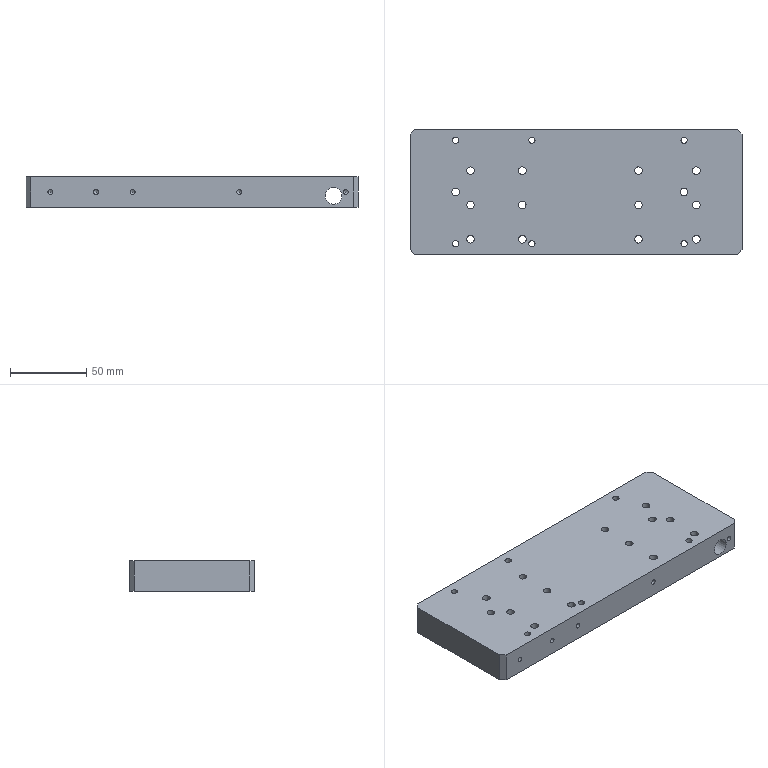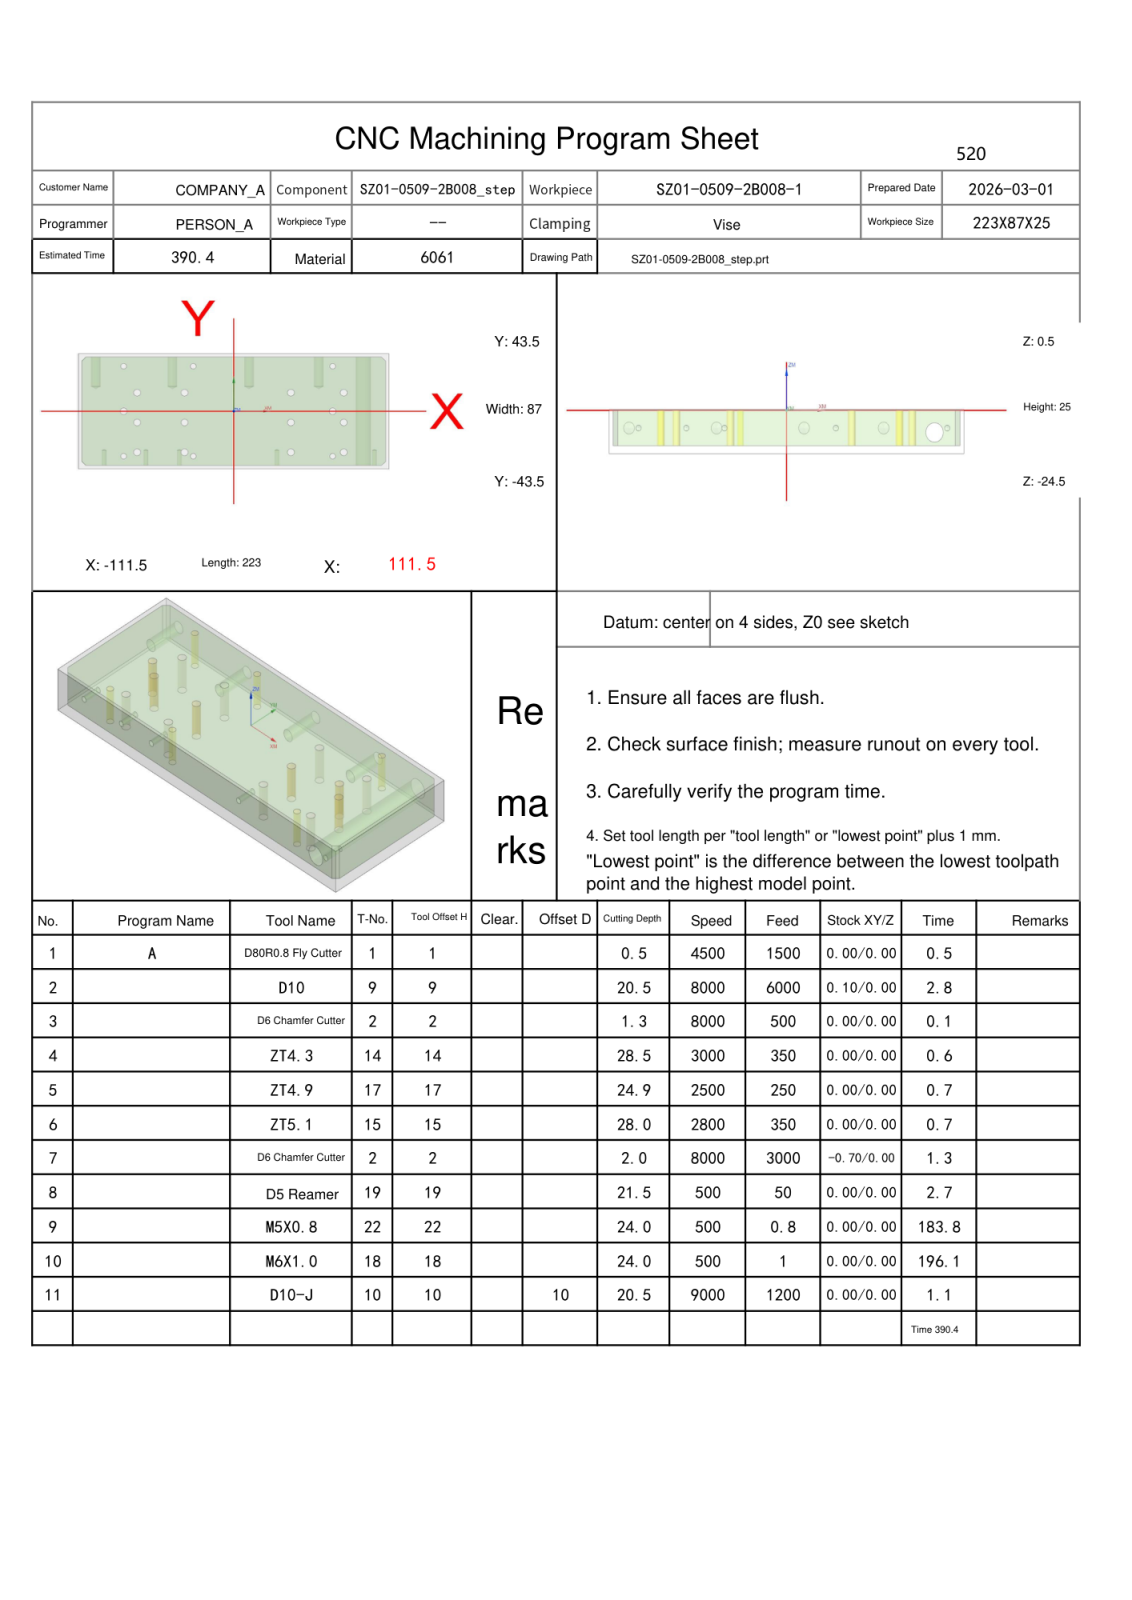NC program | NX | posted by the shop | part box 218 x 82 x 20 mm
Whole program:
%
O0001
(Machine time: 756.44 MIN)
(===Total Tool:10===)
(T1=D80R0.8 Fly Cutter D=80.  R=0.8  D-  H01 Z=0.    )
(T9=D10     D=10.  R=0.   D-  H09 Z=-20.  )
(T2=D6 Chamfer Cutter   D=6.   R=0.   D-  H02 Z=-1.5  )
(T14=ZT4.3  D=4.3  DR_a=118 D-  H14 Z=-28.  )
(T17=ZT4.9  D=4.9  DR_a=120 D-  H17 Z=-24.41)
(T15=ZT5.1  D=5.1  DR_a=118 D-  H15 Z=-27.53)
(T19=D5 Reamer   D=5.   DR_a=180 D-  H19 Z=-21.  )
(T22=M5X0.8 D=4.2  DR_a=180 D-  H22 Z=-23.5 )
(T18=M6X1.0 D=5.   DR_a=180 D-  H18 Z=-23.5 )
(T10=D10-J  D=10.  R=0.   D10 H10 Z=-20.  )
G80 G90 G17 G49 G40
G91 G28 Z0
M01
N1 T01 M06
(D80R0.8 Fly Cutter  D=80. R=0.8 H=01 ce=0.00 di=0.00)
G00 G90 G54 X-154. Y27. M03 S4500
G43 H01 Z50.
M08
Z2.
G01 Z0.0 F1500.
X-149.
X149.
Y-27.
X-149.
X-154.
Z2.
G00 Z50.
G91 G28 Z0.0
M05
M09
G91 G28 Z0.0
M01
N2 T09 M06
(D10  D=10. R=0. H=09 ce=0.10 di=0.00)
G00 G90 G54 X0.0 Y46.1 M03 S8000
G43 H09 Z50.
M08
Z.5
G01 X106. Z.366 F6000.
G02 X109.606 Y44.606 Z.361 I0.0 J-5.1
G01 X112.606 Y41.606 Z.356
G02 X114.1 Y38. Z.351 I-3.606 J-3.606
G01 Y-38. Z.255
G02 X112.606 Y-41.606 Z.25 I-5.1 J0.0
G01 X109.606 Y-44.606 Z.245
G02 X106. Y-46.1 Z.239 I-3.606 J3.606
G01 X-106. Z-.028
G02 X-109.606 Y-44.606 Z-.033 I0.0 J5.1
G01 X-112.606 Y-41.606 Z-.038
G02 X-114.1 Y-38. Z-.043 I3.606 J3.606
G01 Y38. Z-.139
G02 X-112.606 Y41.606 Z-.144 I5.1 J0.0
G01 X-109.606 Y44.606 Z-.15
G02 X-107.242 Y45.946 Z-.153 I3.606 J-3.606
X-106. Y46.1 Z-.155 I1.242 J-4.946
G01 X106. Z-.422
G02 X109.606 Y44.606 Z-.427 I0.0 J-5.1
G01 X112.606 Y41.606 Z-.433
G02 X114.1 Y38. Z-.438 I-3.606 J-3.606
G01 Y-38. Z-.534
G02 X112.606 Y-41.606 Z-.539 I-5.1 J0.0
G01 X109.606 Y-44.606 Z-.544
G02 X106. Y-46.1 Z-.549 I-3.606 J3.606
G01 X-106. Z-.816
G02 X-109.606 Y-44.606 Z-.821 I0.0 J5.1
G01 X-112.606 Y-41.606 Z-.827
G02 X-114.1 Y-38. Z-.832 I3.606 J3.606
G01 Y38. Z-.928
G02 X-112.606 Y41.606 Z-.933 I5.1 J0.0
G01 X-109.606 Y44.606 Z-.938
G02 X-107.242 Y45.946 Z-.942 I3.606 J-3.606
X-106. Y46.1 Z-.943 I1.242 J-4.946
G01 X106. Z-1.211
G02 X109.606 Y44.606 Z-1.216 I0.0 J-5.1
G01 X112.606 Y41.606 Z-1.221
G02 X114.1 Y38. Z-1.226 I-3.606 J-3.606
G01 Y-38. Z-1.322
G02 X112.606 Y-41.606 Z-1.327 I-5.1 J0.0
G01 X109.606 Y-44.606 Z-1.332
G02 X106. Y-46.1 Z-1.337 I-3.606 J3.606
G01 X-106. Z-1.605
G02 X-109.606 Y-44.606 Z-1.61 I0.0 J5.1
G01 X-112.606 Y-41.606 Z-1.615
G02 X-114.1 Y-38. Z-1.62 I3.606 J3.606
G01 Y38. Z-1.716
G02 X-112.606 Y41.606 Z-1.721 I5.1 J0.0
G01 X-109.606 Y44.606 Z-1.727
G02 X-107.242 Y45.946 Z-1.73 I3.606 J-3.606
X-106. Y46.1 Z-1.732 I1.242 J-4.946
G01 X106. Z-1.999
G02 X109.606 Y44.606 Z-2.004 I0.0 J-5.1
G01 X112.606 Y41.606 Z-2.01
G02 X114.1 Y38. Z-2.015 I-3.606 J-3.606
G01 Y-38. Z-2.11
G02 X112.606 Y-41.606 Z-2.115 I-5.1 J0.0
G01 X109.606 Y-44.606 Z-2.121
G02 X106. Y-46.1 Z-2.126 I-3.606 J3.606
G01 X-106. Z-2.393
G02 X-109.606 Y-44.606 Z-2.398 I0.0 J5.1
G01 X-112.606 Y-41.606 Z-2.404
G02 X-114.1 Y-38. Z-2.409 I3.606 J3.606
G01 Y38. Z-2.505
G02 X-112.606 Y41.606 Z-2.51 I5.1 J0.0
G01 X-109.606 Y44.606 Z-2.515
G02 X-107.242 Y45.946 Z-2.519 I3.606 J-3.606
X-106. Y46.1 Z-2.52 I1.242 J-4.946
G01 X106. Z-2.788
G02 X109.606 Y44.606 Z-2.793 I0.0 J-5.1
G01 X112.606 Y41.606 Z-2.798
G02 X114.1 Y38. Z-2.803 I-3.606 J-3.606
G01 Y-38. Z-2.899
G02 X112.606 Y-41.606 Z-2.904 I-5.1 J0.0
G01 X109.606 Y-44.606 Z-2.909
G02 X106. Y-46.1 Z-2.914 I-3.606 J3.606
G01 X-106. Z-3.182
G02 X-109.606 Y-44.606 Z-3.187 I0.0 J5.1
G01 X-112.606 Y-41.606 Z-3.192
G02 X-114.1 Y-38. Z-3.197 I3.606 J3.606
G01 Y38. Z-3.293
G02 X-112.606 Y41.606 Z-3.298 I5.1 J0.0
G01 X-109.606 Y44.606 Z-3.304
G02 X-107.242 Y45.946 Z-3.307 I3.606 J-3.606
X-106. Y46.1 Z-3.309 I1.242 J-4.946
G01 X106. Z-3.576
G02 X109.606 Y44.606 Z-3.581 I0.0 J-5.1
G01 X112.606 Y41.606 Z-3.586
G02 X114.1 Y38. Z-3.591 I-3.606 J-3.606
G01 Y-38. Z-3.687
G02 X112.606 Y-41.606 Z-3.692 I-5.1 J0.0
G01 X109.606 Y-44.606 Z-3.698
G02 X106. Y-46.1 Z-3.703 I-3.606 J3.606
G01 X-106. Z-3.97
G02 X-109.606 Y-44.606 Z-3.975 I0.0 J5.1
G01 X-112.606 Y-41.606 Z-3.981
G02 X-114.1 Y-38. Z-3.986 I3.606 J3.606
G01 Y38. Z-4.082
G02 X-112.606 Y41.606 Z-4.087 I5.1 J0.0
G01 X-109.606 Y44.606 Z-4.092
G02 X-107.242 Y45.946 Z-4.095 I3.606 J-3.606
X-106. Y46.1 Z-4.097 I1.242 J-4.946
G01 X106. Z-4.364
G02 X109.606 Y44.606 Z-4.37 I0.0 J-5.1
G01 X112.606 Y41.606 Z-4.375
G02 X114.1 Y38. Z-4.38 I-3.606 J-3.606
G01 Y-38. Z-4.476
G02 X112.606 Y-41.606 Z-4.481 I-5.1 J0.0
G01 X109.606 Y-44.606 Z-4.486
G02 X106. Y-46.1 Z-4.491 I-3.606 J3.606
G01 X-106. Z-4.759
G02 X-109.606 Y-44.606 Z-4.764 I0.0 J5.1
G01 X-112.606 Y-41.606 Z-4.769
G02 X-114.1 Y-38. Z-4.774 I3.606 J3.606
G01 Y38. Z-4.87
G02 X-112.606 Y41.606 Z-4.875 I5.1 J0.0
G01 X-109.606 Y44.606 Z-4.88
G02 X-107.242 Y45.946 Z-4.884 I3.606 J-3.606
X-106. Y46.1 Z-4.886 I1.242 J-4.946
G01 X106. Z-5.153
G02 X109.606 Y44.606 Z-5.158 I0.0 J-5.1
G01 X112.606 Y41.606 Z-5.163
G02 X114.1 Y38. Z-5.168 I-3.606 J-3.606
G01 Y-38. Z-5.264
G02 X112.606 Y-41.606 Z-5.269 I-5.1 J0.0
G01 X109.606 Y-44.606 Z-5.275
G02 X106. Y-46.1 Z-5.28 I-3.606 J3.606
G01 X-106. Z-5.547
G02 X-109.606 Y-44.606 Z-5.552 I0.0 J5.1
G01 X-112.606 Y-41.606 Z-5.558
G02 X-114.1 Y-38. Z-5.563 I3.606 J3.606
G01 Y38. Z-5.659
G02 X-112.606 Y41.606 Z-5.664 I5.1 J0.0
G01 X-109.606 Y44.606 Z-5.669
G02 X-107.242 Y45.946 Z-5.672 I3.606 J-3.606
X-106. Y46.1 Z-5.674 I1.242 J-4.946
G01 X106. Z-5.941
G02 X109.606 Y44.606 Z-5.946 I0.0 J-5.1
G01 X112.606 Y41.606 Z-5.952
G02 X114.1 Y38. Z-5.957 I-3.606 J-3.606
G01 Y-38. Z-6.053
G02 X112.606 Y-41.606 Z-6.058 I-5.1 J0.0
G01 X109.606 Y-44.606 Z-6.063
G02 X106. Y-46.1 Z-6.068 I-3.606 J3.606
G01 X-106. Z-6.336
G02 X-109.606 Y-44.606 Z-6.341 I0.0 J5.1
G01 X-112.606 Y-41.606 Z-6.346
G02 X-114.1 Y-38. Z-6.351 I3.606 J3.606
G01 Y38. Z-6.447
G02 X-112.606 Y41.606 Z-6.452 I5.1 J0.0
G01 X-109.606 Y44.606 Z-6.457
G02 X-107.242 Y45.946 Z-6.461 I3.606 J-3.606
X-106. Y46.1 Z-6.462 I1.242 J-4.946
G01 X106. Z-6.73
G02 X109.606 Y44.606 Z-6.735 I0.0 J-5.1
G01 X112.606 Y41.606 Z-6.74
G02 X114.1 Y38. Z-6.745 I-3.606 J-3.606
G01 Y-38. Z-6.841
G02 X112.606 Y-41.606 Z-6.846 I-5.1 J0.0
G01 X109.606 Y-44.606 Z-6.852
G02 X106. Y-46.1 Z-6.857 I-3.606 J3.606
G01 X-106. Z-7.124
G02 X-109.606 Y-44.606 Z-7.129 I0.0 J5.1
G01 X-112.606 Y-41.606 Z-7.135
G02 X-114.1 Y-38. Z-7.14 I3.606 J3.606
G01 Y38. Z-7.235
G02 X-112.606 Y41.606 Z-7.24 I5.1 J0.0
G01 X-109.606 Y44.606 Z-7.246
G02 X-107.242 Y45.946 Z-7.249 I3.606 J-3.606
X-106. Y46.1 Z-7.251 I1.242 J-4.946
G01 X106. Z-7.518
G02 X109.606 Y44.606 Z-7.523 I0.0 J-5.1
G01 X112.606 Y41.606 Z-7.529
G02 X114.1 Y38. Z-7.534 I-3.606 J-3.606
G01 Y-38. Z-7.63
G02 X112.606 Y-41.606 Z-7.635 I-5.1 J0.0
G01 X109.606 Y-44.606 Z-7.64
G02 X106. Y-46.1 Z-7.645 I-3.606 J3.606
G01 X-106. Z-7.913
G02 X-109.606 Y-44.606 Z-7.918 I0.0 J5.1
G01 X-112.606 Y-41.606 Z-7.923
G02 X-114.1 Y-38. Z-7.928 I3.606 J3.606
G01 Y38. Z-8.024
G02 X-112.606 Y41.606 Z-8.029 I5.1 J0.0
G01 X-109.606 Y44.606 Z-8.034
G02 X-107.242 Y45.946 Z-8.038 I3.606 J-3.606
X-106. Y46.1 Z-8.039 I1.242 J-4.946
G01 X106. Z-8.307
G02 X109.606 Y44.606 Z-8.312 I0.0 J-5.1
G01 X112.606 Y41.606 Z-8.317
G02 X114.1 Y38. Z-8.322 I-3.606 J-3.606
G01 Y-38. Z-8.418
G02 X112.606 Y-41.606 Z-8.423 I-5.1 J0.0
G01 X109.606 Y-44.606 Z-8.429
G02 X106. Y-46.1 Z-8.434 I-3.606 J3.606
G01 X-106. Z-8.701
G02 X-109.606 Y-44.606 Z-8.706 I0.0 J5.1
G01 X-112.606 Y-41.606 Z-8.711
G02 X-114.1 Y-38. Z-8.716 I3.606 J3.606
G01 Y38. Z-8.812
G02 X-112.606 Y41.606 Z-8.817 I5.1 J0.0
G01 X-109.606 Y44.606 Z-8.823
G02 X-107.242 Y45.946 Z-8.826 I3.606 J-3.606
X-106. Y46.1 Z-8.828 I1.242 J-4.946
G01 X106. Z-9.095
G02 X109.606 Y44.606 Z-9.1 I0.0 J-5.1
G01 X112.606 Y41.606 Z-9.106
G02 X114.1 Y38. Z-9.111 I-3.606 J-3.606
G01 Y-38. Z-9.207
G02 X112.606 Y-41.606 Z-9.212 I-5.1 J0.0
G01 X109.606 Y-44.606 Z-9.217
G02 X106. Y-46.1 Z-9.222 I-3.606 J3.606
G01 X-106. Z-9.489
G02 X-109.606 Y-44.606 Z-9.495 I0.0 J5.1
G01 X-112.606 Y-41.606 Z-9.5
G02 X-114.1 Y-38. Z-9.505 I3.606 J3.606
G01 Y38. Z-9.601
G02 X-112.606 Y41.606 Z-9.606 I5.1 J0.0
G01 X-109.606 Y44.606 Z-9.611
G02 X-107.242 Y45.946 Z-9.615 I3.606 J-3.606
X-106. Y46.1 Z-9.616 I1.242 J-4.946
G01 X106. Z-9.884
G02 X109.606 Y44.606 Z-9.889 I0.0 J-5.1
G01 X112.606 Y41.606 Z-9.894
G02 X114.1 Y38. Z-9.899 I-3.606 J-3.606
G01 Y-38. Z-9.995
G02 X112.606 Y-41.606 Z-10. I-5.1 J0.0
G01 X109.606 Y-44.606 Z-10.005
G02 X106. Y-46.1 Z-10.011 I-3.606 J3.606
G01 X-106. Z-10.278
G02 X-109.606 Y-44.606 Z-10.283 I0.0 J5.1
G01 X-112.606 Y-41.606 Z-10.288
G02 X-114.1 Y-38. Z-10.293 I3.606 J3.606
G01 Y38. Z-10.389
G02 X-112.606 Y41.606 Z-10.394 I5.1 J0.0
G01 X-109.606 Y44.606 Z-10.4
G02 X-107.242 Y45.946 Z-10.403 I3.606 J-3.606
X-106. Y46.1 Z-10.405 I1.242 J-4.946
G01 X106. Z-10.672
G02 X109.606 Y44.606 Z-10.677 I0.0 J-5.1
G01 X112.606 Y41.606 Z-10.683
G02 X114.1 Y38. Z-10.688 I-3.606 J-3.606
G01 Y-38. Z-10.784
G02 X112.606 Y-41.606 Z-10.789 I-5.1 J0.0
G01 X109.606 Y-44.606 Z-10.794
G02 X106. Y-46.1 Z-10.799 I-3.606 J3.606
G01 X-106. Z-11.066
G02 X-109.606 Y-44.606 Z-11.071 I0.0 J5.1
G01 X-112.606 Y-41.606 Z-11.077
G02 X-114.1 Y-38. Z-11.082 I3.606 J3.606
G01 Y38. Z-11.178
G02 X-112.606 Y41.606 Z-11.183 I5.1 J0.0
G01 X-109.606 Y44.606 Z-11.188
G02 X-107.242 Y45.946 Z-11.192 I3.606 J-3.606
X-106. Y46.1 Z-11.193 I1.242 J-4.946
G01 X106. Z-11.461
G02 X109.606 Y44.606 Z-11.466 I0.0 J-5.1
G01 X112.606 Y41.606 Z-11.471
G02 X114.1 Y38. Z-11.476 I-3.606 J-3.606
G01 Y-38. Z-11.572
G02 X112.606 Y-41.606 Z-11.577 I-5.1 J0.0
G01 X109.606 Y-44.606 Z-11.582
G02 X106. Y-46.1 Z-11.587 I-3.606 J3.606
G01 X-106. Z-11.855
G02 X-109.606 Y-44.606 Z-11.86 I0.0 J5.1
G01 X-112.606 Y-41.606 Z-11.865
G02 X-114.1 Y-38. Z-11.87 I3.606 J3.606
G01 Y38. Z-11.966
G02 X-112.606 Y41.606 Z-11.971 I5.1 J0.0
G01 X-109.606 Y44.606 Z-11.977
G02 X-107.242 Y45.946 Z-11.98 I3.606 J-3.606
X-106. Y46.1 Z-11.982 I1.242 J-4.946
G01 X106. Z-12.249
G02 X109.606 Y44.606 Z-12.254 I0.0 J-5.1
G01 X112.606 Y41.606 Z-12.26
G02 X114.1 Y38. Z-12.265 I-3.606 J-3.606
G01 Y-38. Z-12.36
G02 X112.606 Y-41.606 Z-12.365 I-5.1 J0.0
G01 X109.606 Y-44.606 Z-12.371
G02 X106. Y-46.1 Z-12.376 I-3.606 J3.606
G01 X-106. Z-12.643
G02 X-109.606 Y-44.606 Z-12.648 I0.0 J5.1
G01 X-112.606 Y-41.606 Z-12.654
G02 X-114.1 Y-38. Z-12.659 I3.606 J3.606
G01 Y38. Z-12.755
G02 X-112.606 Y41.606 Z-12.76 I5.1 J0.0
G01 X-109.606 Y44.606 Z-12.765
G02 X-107.242 Y45.946 Z-12.769 I3.606 J-3.606
X-106. Y46.1 Z-12.77 I1.242 J-4.946
G01 X106. Z-13.038
G02 X109.606 Y44.606 Z-13.043 I0.0 J-5.1
G01 X112.606 Y41.606 Z-13.048
G02 X114.1 Y38. Z-13.053 I-3.606 J-3.606
G01 Y-38. Z-13.149
G02 X112.606 Y-41.606 Z-13.154 I-5.1 J0.0
G01 X109.606 Y-44.606 Z-13.159
G02 X106. Y-46.1 Z-13.164 I-3.606 J3.606
G01 X-106. Z-13.432
G02 X-109.606 Y-44.606 Z-13.437 I0.0 J5.1
G01 X-112.606 Y-41.606 Z-13.442
G02 X-114.1 Y-38. Z-13.447 I3.606 J3.606
G01 Y38. Z-13.543
G02 X-112.606 Y41.606 Z-13.548 I5.1 J0.0
G01 X-109.606 Y44.606 Z-13.554
G02 X-107.242 Y45.946 Z-13.557 I3.606 J-3.606
X-106. Y46.1 Z-13.559 I1.242 J-4.946
G01 X106. Z-13.826
G02 X109.606 Y44.606 Z-13.831 I0.0 J-5.1
G01 X112.606 Y41.606 Z-13.836
G02 X114.1 Y38. Z-13.841 I-3.606 J-3.606
G01 Y-38. Z-13.937
G02 X112.606 Y-41.606 Z-13.942 I-5.1 J0.0
G01 X109.606 Y-44.606 Z-13.948
G02 X106. Y-46.1 Z-13.953 I-3.606 J3.606
G01 X-106. Z-14.22
G02 X-109.606 Y-44.606 Z-14.225 I0.0 J5.1
G01 X-112.606 Y-41.606 Z-14.231
G02 X-114.1 Y-38. Z-14.236 I3.606 J3.606
G01 Y38. Z-14.332
G02 X-112.606 Y41.606 Z-14.337 I5.1 J0.0
G01 X-109.606 Y44.606 Z-14.342
G02 X-107.242 Y45.946 Z-14.345 I3.606 J-3.606
X-106. Y46.1 Z-14.347 I1.242 J-4.946
G01 X106. Z-14.614
G02 X109.606 Y44.606 Z-14.62 I0.0 J-5.1
G01 X112.606 Y41.606 Z-14.625
G02 X114.1 Y38. Z-14.63 I-3.606 J-3.606
G01 Y-38. Z-14.726
G02 X112.606 Y-41.606 Z-14.731 I-5.1 J0.0
G01 X109.606 Y-44.606 Z-14.736
G02 X106. Y-46.1 Z-14.741 I-3.606 J3.606
G01 X-106. Z-15.009
G02 X-109.606 Y-44.606 Z-15.014 I0.0 J5.1
G01 X-112.606 Y-41.606 Z-15.019
G02 X-114.1 Y-38. Z-15.024 I3.606 J3.606
G01 Y38. Z-15.12
G02 X-112.606 Y41.606 Z-15.125 I5.1 J0.0
G01 X-109.606 Y44.606 Z-15.13
G02 X-107.242 Y45.946 Z-15.134 I3.606 J-3.606
X-106. Y46.1 Z-15.136 I1.242 J-4.946
G01 X106. Z-15.403
G02 X109.606 Y44.606 Z-15.408 I0.0 J-5.1
G01 X112.606 Y41.606 Z-15.413
G02 X114.1 Y38. Z-15.418 I-3.606 J-3.606
G01 Y-38. Z-15.514
G02 X112.606 Y-41.606 Z-15.519 I-5.1 J0.0
G01 X109.606 Y-44.606 Z-15.525
G02 X106. Y-46.1 Z-15.53 I-3.606 J3.606
G01 X-106. Z-15.797
G02 X-109.606 Y-44.606 Z-15.802 I0.0 J5.1
G01 X-112.606 Y-41.606 Z-15.808
G02 X-114.1 Y-38. Z-15.813 I3.606 J3.606
G01 Y38. Z-15.909
G02 X-112.606 Y41.606 Z-15.914 I5.1 J0.0
G01 X-109.606 Y44.606 Z-15.919
G02 X-107.242 Y45.946 Z-15.922 I3.606 J-3.606
X-106. Y46.1 Z-15.924 I1.242 J-4.946
G01 X106. Z-16.191
G02 X109.606 Y44.606 Z-16.196 I0.0 J-5.1
G01 X112.606 Y41.606 Z-16.202
G02 X114.1 Y38. Z-16.207 I-3.606 J-3.606
G01 Y-38. Z-16.303
G02 X112.606 Y-41.606 Z-16.308 I-5.1 J0.0
G01 X109.606 Y-44.606 Z-16.313
G02 X106. Y-46.1 Z-16.318 I-3.606 J3.606
G01 X-106. Z-16.586
G02 X-109.606 Y-44.606 Z-16.591 I0.0 J5.1
G01 X-112.606 Y-41.606 Z-16.596
G02 X-114.1 Y-38. Z-16.601 I3.606 J3.606
G01 Y38. Z-16.697
G02 X-112.606 Y41.606 Z-16.702 I5.1 J0.0
G01 X-109.606 Y44.606 Z-16.707
G02 X-107.242 Y45.946 Z-16.711 I3.606 J-3.606
X-106. Y46.1 Z-16.712 I1.242 J-4.946
G01 X106. Z-16.98
G02 X109.606 Y44.606 Z-16.985 I0.0 J-5.1
G01 X112.606 Y41.606 Z-16.99
G02 X114.1 Y38. Z-16.995 I-3.606 J-3.606
G01 Y-38. Z-17.091
G02 X112.606 Y-41.606 Z-17.096 I-5.1 J0.0
G01 X109.606 Y-44.606 Z-17.102
G02 X106. Y-46.1 Z-17.107 I-3.606 J3.606
G01 X-106. Z-17.374
G02 X-109.606 Y-44.606 Z-17.379 I0.0 J5.1
G01 X-112.606 Y-41.606 Z-17.385
G02 X-114.1 Y-38. Z-17.39 I3.606 J3.606
G01 Y38. Z-17.485
G02 X-112.606 Y41.606 Z-17.49 I5.1 J0.0
G01 X-109.606 Y44.606 Z-17.496
G02 X-107.242 Y45.946 Z-17.499 I3.606 J-3.606
X-106. Y46.1 Z-17.501 I1.242 J-4.946
G01 X106. Z-17.768
G02 X109.606 Y44.606 Z-17.773 I0.0 J-5.1
G01 X112.606 Y41.606 Z-17.779
G02 X114.1 Y38. Z-17.784 I-3.606 J-3.606
G01 Y-38. Z-17.88
G02 X112.606 Y-41.606 Z-17.885 I-5.1 J0.0
G01 X109.606 Y-44.606 Z-17.89
G02 X106. Y-46.1 Z-17.895 I-3.606 J3.606
G01 X-106. Z-18.163
G02 X-109.606 Y-44.606 Z-18.168 I0.0 J5.1
G01 X-112.606 Y-41.606 Z-18.173
G02 X-114.1 Y-38. Z-18.178 I3.606 J3.606
G01 Y38. Z-18.274
G02 X-112.606 Y41.606 Z-18.279 I5.1 J0.0
G01 X-109.606 Y44.606 Z-18.284
G02 X-107.242 Y45.946 Z-18.288 I3.606 J-3.606
X-106. Y46.1 Z-18.289 I1.242 J-4.946
G01 X106. Z-18.557
G02 X109.606 Y44.606 Z-18.562 I0.0 J-5.1
G01 X112.606 Y41.606 Z-18.567
G02 X114.1 Y38. Z-18.572 I-3.606 J-3.606
G01 Y-38. Z-18.668
G02 X112.606 Y-41.606 Z-18.673 I-5.1 J0.0
G01 X109.606 Y-44.606 Z-18.679
G02 X106. Y-46.1 Z-18.684 I-3.606 J3.606
G01 X-106. Z-18.951
G02 X-109.606 Y-44.606 Z-18.956 I0.0 J5.1
G01 X-112.606 Y-41.606 Z-18.961
G02 X-114.1 Y-38. Z-18.966 I3.606 J3.606
G01 Y38. Z-19.062
G02 X-112.606 Y41.606 Z-19.067 I5.1 J0.0
G01 X-109.606 Y44.606 Z-19.073
G02 X-107.242 Y45.946 Z-19.076 I3.606 J-3.606
X-106. Y46.1 Z-19.078 I1.242 J-4.946
G01 X106. Z-19.345
G02 X109.606 Y44.606 Z-19.35 I0.0 J-5.1
G01 X112.606 Y41.606 Z-19.356
G02 X114.1 Y38. Z-19.361 I-3.606 J-3.606
G01 Y-38. Z-19.457
G02 X112.606 Y-41.606 Z-19.462 I-5.1 J0.0
G01 X109.606 Y-44.606 Z-19.467
G02 X106. Y-46.1 Z-19.472 I-3.606 J3.606
G01 X-106. Z-19.739
G02 X-109.606 Y-44.606 Z-19.745 I0.0 J5.1
G01 X-112.606 Y-41.606 Z-19.75
G02 X-114.1 Y-38. Z-19.755 I3.606 J3.606
G01 Y38. Z-19.851
G02 X-112.606 Y41.606 Z-19.856 I5.1 J0.0
G01 X-109.606 Y44.606 Z-19.861
G02 X-107.242 Y45.946 Z-19.865 I3.606 J-3.606
X-106. Y46.1 Z-19.866 I1.242 J-4.946
G01 X0.0 Z-20.
X106.
G02 X109.606 Y44.606 I0.0 J-5.1
G01 X112.606 Y41.606
G02 X114.1 Y38. I-3.606 J-3.606
G01 Y-38.
G02 X112.606 Y-41.606 I-5.1 J0.0
G01 X109.606 Y-44.606
G02 X106. Y-46.1 I-3.606 J3.606
G01 X-106.
G02 X-109.606 Y-44.606 I0.0 J5.1
G01 X-112.606 Y-41.606
G02 X-114.1 Y-38. I3.606 J3.606
G01 Y38.
G02 X-112.606 Y41.606 I5.1 J0.0
G01 X-109.606 Y44.606
G02 X-106. Y46.1 I3.606 J-3.606
G01 X0.0
X.5
Z-19.
G00 Z50.
G91 G28 Z0.0
M05
M09
G91 G28 Z0.0
M01
N3 T02 M06
(D6 Chamfer Cutter  D=6. R=0. H=02 ce=0.00 di=0.00)
G00 G90 G54 X71. Y34. M03 S8000
G43 H02 Z50.
M08
G98 G81 X71. Y34. Z-.8 R1. F500.
X79. Y14.
X71. Y0.0
X79. Y-8.5
Y-31.
X71. Y-34.
X41. Y-31.
Y-8.5
Y14.
X-29. Y34.
X-35.275 Y14.
Y-8.5
X-29. Y-34.
X-35.275 Y-31.
X-69.275
X-79. Y-34.
X-69.275 Y-8.5
X-79. Y0.0
X-69.275 Y14.
X-79. Y34.
G80
G00 Z50.
G91 G28 Z0.0
M05
M09
G91 G28 Z0.0
M01
N4 T14 M06
(ZT4.3 D=4.3 DR_a=118 H=14)
G00 G90 G54 X-29. Y-34. M03 S3000
G43 H14 Z50.
M08
G98 G83 X-29. Y-34. Z-28. R1. F350. Q3.
X-79.
Y34.
X-29.
X71.
Y-34.
G80
G00 Z50.
G91 G28 Z0.0
M05
M09
G91 G28 Z0.0
M01
N5 T17 M06
(ZT4.9 D=4.9 DR_a=120 H=17)
G00 G90 G54 X-79. Y0.0 M03 S2500
G43 H17 Z50.
M08
G98 G83 X-79. Y0.0 Z-24.415 R1. F250. Q2.
X-69.275 Y-8.5
X-35.275
X41.
X71. Y0.0
X79. Y-8.5
G80
G00 Z50.
G91 G28 Z0.0
M05
M09
G91 G28 Z0.0
M01
N6 T15 M06
(ZT5.1 D=5.1 DR_a=118 H=15)
G00 G90 G54 X41. Y-31. M03 S2800
G43 H15 Z50.
M08
G98 G83 X41. Y-31. Z-27.532 R1. F350. Q3.
X79.
Y14.
X41.
X-35.275
X-69.275
Y-31.
X-35.275
G80
G00 Z50.
G91 G28 Z0.0
M05
M09
G91 G28 Z0.0
M01
N7 T02 M06
(D6 Chamfer Cutter  D=6. R=0. H=02 ce=0.00 di=0.00)
G00 G90 G54 X-.25 Y43.128 M03 S8000
G43 H02 Z50.
M08
Z2.099
G01 Z-1.5 F3000.
G03 X-.33 Y42.828 I.52 J-.3
X-.03 Y42.308 I.6 J0.0
G01 X0.0 Y42.3
X106.
X106.254 Y42.275
X106.497 Y42.201
X106.722 Y42.081
X106.919 Y41.919
X109.919 Y38.919
X110.081 Y38.722
X110.201 Y38.497
X110.275 Y38.254
X110.3 Y38.
Y-38.
X110.275 Y-38.254
X110.201 Y-38.497
X110.081 Y-38.722
X109.919 Y-38.919
X106.919 Y-41.919
X106.722 Y-42.081
X106.497 Y-42.201
X106.254 Y-42.275
X106. Y-42.3
X-106.
X-106.254 Y-42.275
X-106.497 Y-42.201
X-106.722 Y-42.081
X-106.919 Y-41.919
X-109.919 Y-38.919
X-110.081 Y-38.722
X-110.201 Y-38.497
X-110.275 Y-38.254
X-110.3 Y-38.
Y38.
X-110.275 Y38.254
X-110.201 Y38.497
X-110.081 Y38.722
X-109.919 Y38.919
X-106.919 Y41.919
X-106.722 Y42.081
X-106.497 Y42.201
X-106.254 Y42.275
X-106. Y42.3
X0.0
X.03 Y42.308
G03 X.33 Y42.828 I-.3 J.52
X.25 Y43.128 I-.6 J0.0
G01 Z2.099
G00 Z50.
G00 G90 X-28.907 Y33.306 M03 S8000
Z50.
Z-.5
G01 Z-1. F500.
X-28.8 Y32.5
G03 X-27.3 Y34. I0.0 J1.5
X-29. Y35.7 I-1.7 J0.0
X-30.7 Y34. I0.0 J-1.7
X-29. Y32.3 I1.7 J0.0
X-27.3 Y34. I0.0 J1.7
X-28.8 Y35.5 I-1.5 J0.0
G01 X-28.907 Y34.694
Z-.5
G00 Z50.
X-78.907 Y33.306
Z-.5
G01 Z-1.
X-78.8 Y32.5
G03 X-77.3 Y34. I0.0 J1.5
X-79. Y35.7 I-1.7 J0.0
X-80.7 Y34. I0.0 J-1.7
X-79. Y32.3 I1.7 J0.0
X-77.3 Y34. I0.0 J1.7
X-78.8 Y35.5 I-1.5 J0.0
G01 X-78.907 Y34.694
Z-.5
G00 Z50.
Y-34.694
Z-.5
G01 Z-1.
X-78.8 Y-35.5
G03 X-77.3 Y-34. I0.0 J1.5
X-79. Y-32.3 I-1.7 J0.0
X-80.7 Y-34. I0.0 J-1.7
X-79. Y-35.7 I1.7 J0.0
X-77.3 Y-34. I0.0 J1.7
X-78.8 Y-32.5 I-1.5 J0.0
G01 X-78.907 Y-33.306
Z-.5
G00 Z50.
X-28.907 Y-34.694
Z-.5
G01 Z-1.
X-28.8 Y-35.5
G03 X-27.3 Y-34. I0.0 J1.5
X-29. Y-32.3 I-1.7 J0.0
X-30.7 Y-34. I0.0 J-1.7
X-29. Y-35.7 I1.7 J0.0
X-27.3 Y-34. I0.0 J1.7
X-28.8 Y-32.5 I-1.5 J0.0
G01 X-28.907 Y-33.306
Z-.5
G00 Z50.
X71.093 Y-34.694
Z-.5
G01 Z-1.
X71.2 Y-35.5
G03 X72.7 Y-34. I0.0 J1.5
X71. Y-32.3 I-1.7 J0.0
X69.3 Y-34. I0.0 J-1.7
X71. Y-35.7 I1.7 J0.0
X72.7 Y-34. I0.0 J1.7
X71.2 Y-32.5 I-1.5 J0.0
G01 X71.093 Y-33.306
Z-.5
G00 Z50.
Y33.306
Z-.5
G01 Z-1.
X71.2 Y32.5
G03 X72.7 Y34. I0.0 J1.5
X71. Y35.7 I-1.7 J0.0
X69.3 Y34. I0.0 J-1.7
X71. Y32.3 I1.7 J0.0
X72.7 Y34. I0.0 J1.7
X71.2 Y35.5 I-1.5 J0.0
G01 X71.093 Y34.694
Z-.5
G00 Z50.
G00 G90 X79.157 Y-9.284 M03 S8000
Z50.
Z-.5
G01 Z-1. F500.
X79.3 Y-10.
G03 X80.8 Y-8.5 I0.0 J1.5
X79. Y-6.7 I-1.8 J0.0
X77.2 Y-8.5 I0.0 J-1.8
X79. Y-10.3 I1.8 J0.0
X80.8 Y-8.5 I0.0 J1.8
X79.3 Y-7. I-1.5 J0.0
G01 X79.157 Y-7.716
Z-.5
G00 Z50.
X71.157 Y-.784
Z-.5
G01 Z-1.
X71.3 Y-1.5
G03 X72.8 Y0.0 I0.0 J1.5
X71. Y1.8 I-1.8 J0.0
X69.2 Y0.0 I0.0 J-1.8
X71. Y-1.8 I1.8 J0.0
X72.8 Y0.0 I0.0 J1.8
X71.3 Y1.5 I-1.5 J0.0
G01 X71.157 Y.784
Z-.5
G00 Z50.
X41.157 Y-9.284
Z-.5
G01 Z-1.
X41.3 Y-10.
G03 X42.8 Y-8.5 I0.0 J1.5
X41. Y-6.7 I-1.8 J0.0
X39.2 Y-8.5 I0.0 J-1.8
X41. Y-10.3 I1.8 J0.0
X42.8 Y-8.5 I0.0 J1.8
X41.3 Y-7. I-1.5 J0.0
G01 X41.157 Y-7.716
Z-.5
G00 Z50.
X-35.118 Y-9.284
Z-.5
G01 Z-1.
X-34.975 Y-10.
G03 X-33.475 Y-8.5 I0.0 J1.5
X-35.275 Y-6.7 I-1.8 J0.0
X-37.075 Y-8.5 I0.0 J-1.8
X-35.275 Y-10.3 I1.8 J0.0
X-33.475 Y-8.5 I0.0 J1.8
X-34.975 Y-7. I-1.5 J0.0
G01 X-35.118 Y-7.716
Z-.5
G00 Z50.
X-69.118 Y-9.284
Z-.5
G01 Z-1.
X-68.975 Y-10.
G03 X-67.475 Y-8.5 I0.0 J1.5
X-69.275 Y-6.7 I-1.8 J0.0
X-71.075 Y-8.5 I0.0 J-1.8
X-69.275 Y-10.3 I1.8 J0.0
X-67.475 Y-8.5 I0.0 J1.8
X-68.975 Y-7. I-1.5 J0.0
G01 X-69.118 Y-7.716
Z-.5
G00 Z50.
X-78.843 Y-.784
Z-.5
G01 Z-1.
X-78.7 Y-1.5
G03 X-77.2 Y0.0 I0.0 J1.5
X-79. Y1.8 I-1.8 J0.0
X-80.8 Y0.0 I0.0 J-1.8
X-79. Y-1.8 I1.8 J0.0
X-77.2 Y0.0 I0.0 J1.8
X-78.7 Y1.5 I-1.5 J0.0
G01 X-78.843 Y.784
Z-.5
G00 Z50.
G00 G90 X-34.818 Y12.945 M03 S8000
Z50.
Z-.6
G01 Z-1.1 F500.
X-34.625 Y12.5
G03 X-33.125 Y14. I0.0 J1.5
X-35.275 Y16.15 I-2.15 J0.0
X-37.425 Y14. I0.0 J-2.15
X-35.275 Y11.85 I2.15 J0.0
X-33.125 Y14. I0.0 J2.15
X-34.625 Y15.5 I-1.5 J0.0
G01 X-34.818 Y15.055
Z-.6
G00 Z50.
X-68.818 Y12.945
Z-.6
G01 Z-1.1
X-68.625 Y12.5
G03 X-67.125 Y14. I0.0 J1.5
X-69.275 Y16.15 I-2.15 J0.0
X-71.425 Y14. I0.0 J-2.15
X-69.275 Y11.85 I2.15 J0.0
X-67.125 Y14. I0.0 J2.15
X-68.625 Y15.5 I-1.5 J0.0
G01 X-68.818 Y15.055
Z-.6
G00 Z50.
Y-32.055
Z-.6
G01 Z-1.1
X-68.625 Y-32.5
G03 X-67.125 Y-31. I0.0 J1.5
X-69.275 Y-28.85 I-2.15 J0.0
X-71.425 Y-31. I0.0 J-2.15
X-69.275 Y-33.15 I2.15 J0.0
X-67.125 Y-31. I0.0 J2.15
X-68.625 Y-29.5 I-1.5 J0.0
G01 X-68.818 Y-29.945
Z-.6
G00 Z50.
X-34.818 Y-32.055
Z-.6
G01 Z-1.1
X-34.625 Y-32.5
G03 X-33.125 Y-31. I0.0 J1.5
X-35.275 Y-28.85 I-2.15 J0.0
X-37.425 Y-31. I0.0 J-2.15
X-35.275 Y-33.15 I2.15 J0.0
X-33.125 Y-31. I0.0 J2.15
X-34.625 Y-29.5 I-1.5 J0.0
G01 X-34.818 Y-29.945
Z-.6
G00 Z50.
X41.457 Y-32.055
Z-.6
G01 Z-1.1
X41.65 Y-32.5
G03 X43.15 Y-31. I0.0 J1.5
X41. Y-28.85 I-2.15 J0.0
X38.85 Y-31. I0.0 J-2.15
X41. Y-33.15 I2.15 J0.0
X43.15 Y-31. I0.0 J2.15
X41.65 Y-29.5 I-1.5 J0.0
G01 X41.457 Y-29.945
Z-.6
G00 Z50.
X79.457 Y-32.055
Z-.6
G01 Z-1.1
X79.65 Y-32.5
G03 X81.15 Y-31. I0.0 J1.5
X79. Y-28.85 I-2.15 J0.0
X76.85 Y-31. I0.0 J-2.15
X79. Y-33.15 I2.15 J0.0
X81.15 Y-31. I0.0 J2.15
X79.65 Y-29.5 I-1.5 J0.0
G01 X79.457 Y-29.945
Z-.6
G00 Z50.
Y12.945
Z-.6
G01 Z-1.1
X79.65 Y12.5
G03 X81.15 Y14. I0.0 J1.5
X79. Y16.15 I-2.15 J0.0
X76.85 Y14. I0.0 J-2.15
X79. Y11.85 I2.15 J0.0
X81.15 Y14. I0.0 J2.15
X79.65 Y15.5 I-1.5 J0.0
G01 X79.457 Y15.055
Z-.6
G00 Z50.
X41.457 Y12.945
Z-.6
G01 Z-1.1
X41.65 Y12.5
G03 X43.15 Y14. I0.0 J1.5
X41. Y16.15 I-2.15 J0.0
X38.85 Y14. I0.0 J-2.15
X41. Y11.85 I2.15 J0.0
X43.15 Y14. I0.0 J2.15
X41.65 Y15.5 I-1.5 J0.0
G01 X41.457 Y15.055
Z-.6
G00 Z50.
G91 G28 Z0.0
M05
M09
G91 G28 Z0.0
M01
N8 T19 M06
(D5 Reamer D=5. DR_a=180 H=19)
G00 G90 G54 X-79. Y0.0 M03 S500
G43 H19 Z50.
M08
G98 G85 X-79. Y0.0 Z-21. R1. F50.
X-69.275 Y-8.5
X-35.275
X41.
X71. Y0.0
X79. Y-8.5
G80
G00 Z50.
G91 G28 Z0.0
M05
M09
G91 G28 Z0.0
M01
N9 T22 M06
(M5X0.8 D=4.2 DR_a=180 H=22)
G00 G90 G54 X-29. Y-34. M03 S500
G43 H22 Z50.
M08
G95
G98 G84 X-29. Y-34. Z-23.5 R1. F.8 Q3.
X-79.
Y34.
X-29.
X71.
Y-34.
G80
G94
G00 Z50.
G91 G28 Z0.0
M05
M09
G91 G28 Z0.0
M01
N10 T18 M06
(M6X1.0 D=5. DR_a=180 H=18)
G00 G90 G54 X41. Y-31. M03 S500
G43 H18 Z50.
M08
G95
G98 G84 X41. Y-31. Z-23.5 R1. F1. Q3.
X79.
Y14.
X41.
X-35.275
X-69.275
Y-31.
X-35.275
G80
G94
G00 Z50.
G91 G28 Z0.0
M05
M09
G91 G28 Z0.0
M01
N11 T10 M06
(D10-J  D=10. R=0. H=10 ce=0.00 di=0.00)
G00 G90 G54 X-107.013 Y47.116 M03 S9000
G43 H10 Z50.
M08
Z-9.5
G01 Z-10. F1200.
G41 D10
X-106.997 Y46.917
G03 X-106. Y46. I.997 J.083
G01 X106.
G02 X109.536 Y44.536 I0.0 J-5.
G01 X112.536 Y41.536
G02 X114. Y38. I-3.536 J-3.536
G01 Y-38.
G02 X112.536 Y-41.536 I-5. J0.0
G01 X109.536 Y-44.536
G02 X106. Y-46. I-3.536 J3.536
G01 X-106.
G02 X-109.536 Y-44.536 I0.0 J5.
G01 X-112.536 Y-41.536
G02 X-114. Y-38. I3.536 J3.536
G01 Y38.
G02 X-112.536 Y41.536 I5. J0.0
G01 X-109.536 Y44.536
G02 X-106. Y46. I3.536 J-3.536
G01 X-105.5
G03 X-104.5 Y47. I0.0 J1.
G01 G40 Y47.2
Z-9.5
G00 Z50.
X-107.013 Y47.116
Z-19.5
G01 Z-20.
G41 D10
X-106.997 Y46.917
G03 X-106. Y46. I.997 J.083
G01 X106.
G02 X109.536 Y44.536 I0.0 J-5.
G01 X112.536 Y41.536
G02 X114. Y38. I-3.536 J-3.536
G01 Y-38.
G02 X112.536 Y-41.536 I-5. J0.0
G01 X109.536 Y-44.536
G02 X106. Y-46. I-3.536 J3.536
G01 X-106.
G02 X-109.536 Y-44.536 I0.0 J5.
G01 X-112.536 Y-41.536
G02 X-114. Y-38. I3.536 J3.536
G01 Y38.
G02 X-112.536 Y41.536 I5. J0.0
G01 X-109.536 Y44.536
G02 X-106. Y46. I3.536 J-3.536
G01 X-105.5
G03 X-104.5 Y47. I0.0 J1.
G01 G40 Y47.2
Z-19.5
G00 Z50.
M05
M09
G91 G28 Z0.0
G91 G28 Y0.0
M30
%